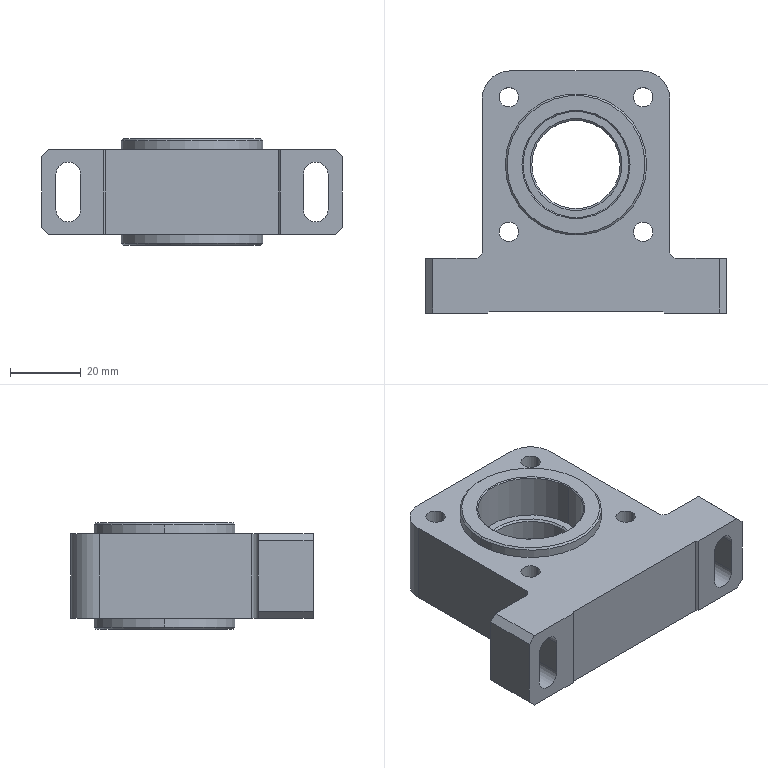Part | STEP file | 04轴承座 EDA50-L_R04-004-BZ^EDA50-R04 (D60N) | 1 solid | 96 faces | box 85 x 68.5 x 30 mm | volume 78011 mm3 | cylinder 44 | plane 30 | cone 22 | commonest cylinder face diameters 3.3 x10 5.5 x8 9 x8 7 x4 30 x4 40 x4